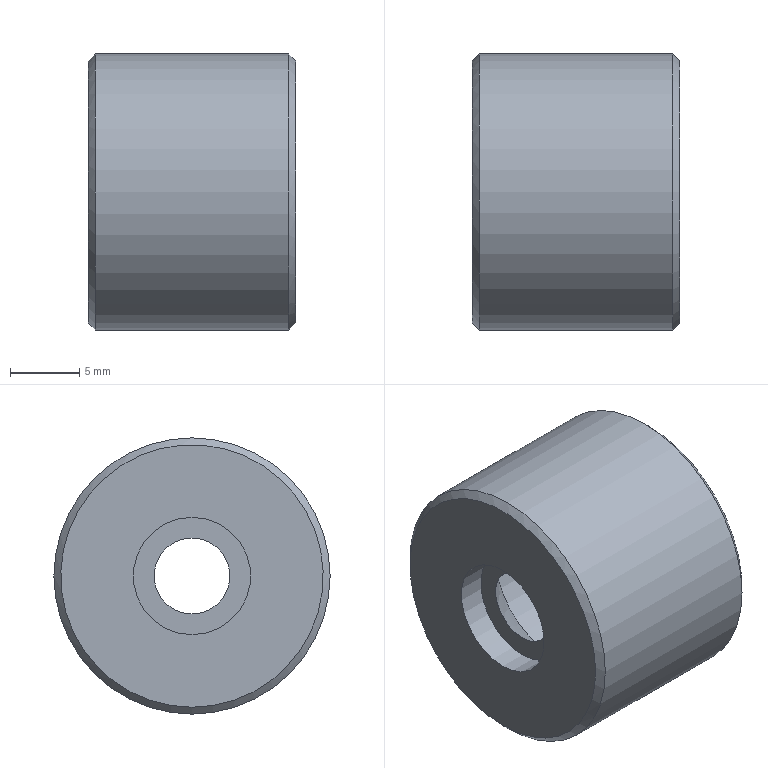Part | NX | features BREP 1 | 1 solid | 12 faces | box 15 x 20 x 20 mm | volume 3272 mm3 | cylinder 4 | plane 4 | cone 4 | commonest cylinder face diameters 5.5 x1 8.5 x1 12 x1 20 x1
STEP:
#1=CARTESIAN_POINT('',(2.015,0.,-2.75));
#2=VERTEX_POINT('',#1);
#3=CARTESIAN_POINT('',(2.015,0.,0.));
#4=DIRECTION('',(1.,0.,0.));
#5=DIRECTION('',(0.,0.,-1.));
#6=AXIS2_PLACEMENT_3D('',#3,#4,#5);
#7=CIRCLE('',#6,2.75);
#8=EDGE_CURVE('',#2,#2,#7,.T.);
#9=ORIENTED_EDGE('',*,*,#8,.T.);
#10=EDGE_LOOP('',(#9));
#11=FACE_BOUND('',#10,.T.);
#12=CARTESIAN_POINT('',(2.,0.,2.75));
#13=VERTEX_POINT('',#12);
#14=CARTESIAN_POINT('',(2.,0.,0.));
#15=DIRECTION('',(1.,0.,0.));
#16=DIRECTION('',(0.,0.,1.));
#17=AXIS2_PLACEMENT_3D('',#14,#15,#16);
#18=CIRCLE('',#17,2.75);
#19=EDGE_CURVE('',#13,#13,#18,.T.);
#20=ORIENTED_EDGE('',*,*,#19,.F.);
#21=EDGE_LOOP('',(#20));
#22=FACE_BOUND('',#21,.T.);
#23=CARTESIAN_POINT('',(5.,0.,0.));
#24=DIRECTION('',(1.,0.,0.));
#25=DIRECTION('',(0.,0.,1.));
#26=AXIS2_PLACEMENT_3D('',#23,#24,#25);
#27=CYLINDRICAL_SURFACE('',#26,2.75);
#28=ADVANCED_FACE('',(#11,#22),#27,.F.);
#29=CARTESIAN_POINT('',(0.,0.,4.25));
#30=VERTEX_POINT('',#29);
#31=CARTESIAN_POINT('',(0.,0.,0.));
#32=DIRECTION('',(-1.,0.,0.));
#33=DIRECTION('',(0.,0.,1.));
#34=AXIS2_PLACEMENT_3D('',#31,#32,#33);
#35=CIRCLE('',#34,4.25);
#36=EDGE_CURVE('',#30,#30,#35,.T.);
#37=ORIENTED_EDGE('',*,*,#36,.F.);
#38=EDGE_LOOP('',(#37));
#39=FACE_BOUND('',#38,.T.);
#40=CARTESIAN_POINT('',(0.,0.,-9.5));
#41=VERTEX_POINT('',#40);
#42=CARTESIAN_POINT('',(0.,0.,0.));
#43=DIRECTION('',(-1.,0.,0.));
#44=DIRECTION('',(0.,0.,-1.));
#45=AXIS2_PLACEMENT_3D('',#42,#43,#44);
#46=CIRCLE('',#45,9.5);
#47=EDGE_CURVE('',#41,#41,#46,.T.);
#48=ORIENTED_EDGE('',*,*,#47,.T.);
#49=EDGE_LOOP('',(#48));
#50=FACE_BOUND('',#49,.T.);
#51=CARTESIAN_POINT('',(0.,10.,0.));
#52=DIRECTION('',(1.,0.,0.));
#53=DIRECTION('',(0.,0.,1.));
#54=AXIS2_PLACEMENT_3D('',#51,#52,#53);
#55=PLANE('',#54);
#56=ADVANCED_FACE('',(#39,#50),#55,.F.);
#57=CARTESIAN_POINT('',(5.,0.,-5.735));
#58=VERTEX_POINT('',#57);
#59=CARTESIAN_POINT('',(5.,0.,0.));
#60=DIRECTION('',(1.,0.,0.));
#61=DIRECTION('',(0.,0.,-1.));
#62=AXIS2_PLACEMENT_3D('',#59,#60,#61);
#63=CIRCLE('',#62,5.735);
#64=EDGE_CURVE('',#58,#58,#63,.T.);
#65=ORIENTED_EDGE('',*,*,#64,.F.);
#66=EDGE_LOOP('',(#65));
#67=FACE_BOUND('',#66,.T.);
#68=CARTESIAN_POINT('',(5.,0.,6.));
#69=VERTEX_POINT('',#68);
#70=CARTESIAN_POINT('',(5.,0.,0.));
#71=DIRECTION('',(-1.,0.,0.));
#72=DIRECTION('',(0.,0.,1.));
#73=AXIS2_PLACEMENT_3D('',#70,#71,#72);
#74=CIRCLE('',#73,6.);
#75=EDGE_CURVE('',#69,#69,#74,.T.);
#76=ORIENTED_EDGE('',*,*,#75,.F.);
#77=EDGE_LOOP('',(#76));
#78=FACE_BOUND('',#77,.T.);
#79=CARTESIAN_POINT('',(5.,0.,0.));
#80=DIRECTION('',(-1.,0.,0.));
#81=DIRECTION('',(0.,0.,-1.));
#82=AXIS2_PLACEMENT_3D('',#79,#80,#81);
#83=PLANE('',#82);
#84=ADVANCED_FACE('',(#67,#78),#83,.F.);
#85=CARTESIAN_POINT('',(14.5,0.,6.));
#86=VERTEX_POINT('',#85);
#87=CARTESIAN_POINT('',(14.5,0.,0.));
#88=DIRECTION('',(1.,0.,0.));
#89=DIRECTION('',(0.,0.,1.));
#90=AXIS2_PLACEMENT_3D('',#87,#88,#89);
#91=CIRCLE('',#90,6.);
#92=EDGE_CURVE('',#86,#86,#91,.T.);
#93=ORIENTED_EDGE('',*,*,#92,.T.);
#94=EDGE_LOOP('',(#93));
#95=FACE_BOUND('',#94,.T.);
#96=ORIENTED_EDGE('',*,*,#75,.T.);
#97=EDGE_LOOP('',(#96));
#98=FACE_BOUND('',#97,.T.);
#99=CARTESIAN_POINT('',(0.,0.,0.));
#100=DIRECTION('',(-1.,0.,0.));
#101=DIRECTION('',(0.,0.,-1.));
#102=AXIS2_PLACEMENT_3D('',#99,#100,#101);
#103=CYLINDRICAL_SURFACE('',#102,6.);
#104=ADVANCED_FACE('',(#95,#98),#103,.F.);
#105=CARTESIAN_POINT('',(15.,0.,6.5));
#106=VERTEX_POINT('',#105);
#107=CARTESIAN_POINT('',(15.,0.,0.));
#108=DIRECTION('',(-1.,0.,0.));
#109=DIRECTION('',(0.,0.,1.));
#110=AXIS2_PLACEMENT_3D('',#107,#108,#109);
#111=CIRCLE('',#110,6.5);
#112=EDGE_CURVE('',#106,#106,#111,.T.);
#113=ORIENTED_EDGE('',*,*,#112,.T.);
#114=EDGE_LOOP('',(#113));
#115=FACE_BOUND('',#114,.T.);
#116=CARTESIAN_POINT('',(15.,0.,9.5));
#117=VERTEX_POINT('',#116);
#118=CARTESIAN_POINT('',(15.,0.,0.));
#119=DIRECTION('',(1.,0.,0.));
#120=DIRECTION('',(0.,0.,1.));
#121=AXIS2_PLACEMENT_3D('',#118,#119,#120);
#122=CIRCLE('',#121,9.5);
#123=EDGE_CURVE('',#117,#117,#122,.T.);
#124=ORIENTED_EDGE('',*,*,#123,.T.);
#125=EDGE_LOOP('',(#124));
#126=FACE_BOUND('',#125,.T.);
#127=CARTESIAN_POINT('',(15.,6.,0.));
#128=DIRECTION('',(-1.,0.,0.));
#129=DIRECTION('',(0.,0.,-1.));
#130=AXIS2_PLACEMENT_3D('',#127,#128,#129);
#131=PLANE('',#130);
#132=ADVANCED_FACE('',(#115,#126),#131,.F.);
#133=CARTESIAN_POINT('',(14.5,0.,10.));
#134=VERTEX_POINT('',#133);
#135=CARTESIAN_POINT('',(14.5,0.,0.));
#136=DIRECTION('',(-1.,0.,0.));
#137=DIRECTION('',(0.,0.,1.));
#138=AXIS2_PLACEMENT_3D('',#135,#136,#137);
#139=CIRCLE('',#138,10.);
#140=EDGE_CURVE('',#134,#134,#139,.T.);
#141=ORIENTED_EDGE('',*,*,#140,.T.);
#142=EDGE_LOOP('',(#141));
#143=FACE_BOUND('',#142,.T.);
#144=CARTESIAN_POINT('',(0.5,0.,-10.));
#145=VERTEX_POINT('',#144);
#146=CARTESIAN_POINT('',(0.5,0.,0.));
#147=DIRECTION('',(1.,0.,0.));
#148=DIRECTION('',(0.,0.,-1.));
#149=AXIS2_PLACEMENT_3D('',#146,#147,#148);
#150=CIRCLE('',#149,10.);
#151=EDGE_CURVE('',#145,#145,#150,.T.);
#152=ORIENTED_EDGE('',*,*,#151,.T.);
#153=EDGE_LOOP('',(#152));
#154=FACE_BOUND('',#153,.T.);
#155=CARTESIAN_POINT('',(0.,0.,0.));
#156=DIRECTION('',(-1.,0.,0.));
#157=DIRECTION('',(0.,0.,-1.));
#158=AXIS2_PLACEMENT_3D('',#155,#156,#157);
#159=CYLINDRICAL_SURFACE('',#158,10.);
#160=ADVANCED_FACE('',(#143,#154),#159,.T.);
#161=ORIENTED_EDGE('',*,*,#92,.F.);
#162=EDGE_LOOP('',(#161));
#163=FACE_BOUND('',#162,.T.);
#164=ORIENTED_EDGE('',*,*,#112,.F.);
#165=EDGE_LOOP('',(#164));
#166=FACE_BOUND('',#165,.T.);
#167=CARTESIAN_POINT('',(15.,0.,0.));
#168=DIRECTION('',(1.,0.,0.));
#169=DIRECTION('',(0.,0.,1.));
#170=AXIS2_PLACEMENT_3D('',#167,#168,#169);
#171=CONICAL_SURFACE('',#170,6.5,0.7854);
#172=ADVANCED_FACE('',(#163,#166),#171,.F.);
#173=ORIENTED_EDGE('',*,*,#123,.F.);
#174=EDGE_LOOP('',(#173));
#175=FACE_BOUND('',#174,.T.);
#176=ORIENTED_EDGE('',*,*,#140,.F.);
#177=EDGE_LOOP('',(#176));
#178=FACE_BOUND('',#177,.T.);
#179=CARTESIAN_POINT('',(14.5,0.,0.));
#180=DIRECTION('',(-1.,0.,0.));
#181=DIRECTION('',(0.,0.,-1.));
#182=AXIS2_PLACEMENT_3D('',#179,#180,#181);
#183=CONICAL_SURFACE('',#182,10.,0.7854);
#184=ADVANCED_FACE('',(#175,#178),#183,.T.);
#185=ORIENTED_EDGE('',*,*,#151,.F.);
#186=EDGE_LOOP('',(#185));
#187=FACE_BOUND('',#186,.T.);
#188=ORIENTED_EDGE('',*,*,#47,.F.);
#189=EDGE_LOOP('',(#188));
#190=FACE_BOUND('',#189,.T.);
#191=CARTESIAN_POINT('',(0.,0.,0.));
#192=DIRECTION('',(1.,0.,0.));
#193=DIRECTION('',(0.,0.,1.));
#194=AXIS2_PLACEMENT_3D('',#191,#192,#193);
#195=CONICAL_SURFACE('',#194,9.5,0.7854);
#196=ADVANCED_FACE('',(#187,#190),#195,.T.);
#197=ORIENTED_EDGE('',*,*,#8,.F.);
#198=EDGE_LOOP('',(#197));
#199=FACE_BOUND('',#198,.T.);
#200=ORIENTED_EDGE('',*,*,#64,.T.);
#201=EDGE_LOOP('',(#200));
#202=FACE_BOUND('',#201,.T.);
#203=CARTESIAN_POINT('',(5.,0.,0.));
#204=DIRECTION('',(1.,0.,0.));
#205=DIRECTION('',(0.,0.,1.));
#206=AXIS2_PLACEMENT_3D('',#203,#204,#205);
#207=CONICAL_SURFACE('',#206,5.735,0.7854);
#208=ADVANCED_FACE('',(#199,#202),#207,.F.);
#209=CARTESIAN_POINT('',(2.,0.,4.25));
#210=VERTEX_POINT('',#209);
#211=CARTESIAN_POINT('',(2.,0.,0.));
#212=DIRECTION('',(-1.,0.,0.));
#213=DIRECTION('',(0.,0.,1.));
#214=AXIS2_PLACEMENT_3D('',#211,#212,#213);
#215=CIRCLE('',#214,4.25);
#216=EDGE_CURVE('',#210,#210,#215,.T.);
#217=ORIENTED_EDGE('',*,*,#216,.T.);
#218=EDGE_LOOP('',(#217));
#219=FACE_BOUND('',#218,.T.);
#220=ORIENTED_EDGE('',*,*,#19,.T.);
#221=EDGE_LOOP('',(#220));
#222=FACE_BOUND('',#221,.T.);
#223=CARTESIAN_POINT('',(2.,0.,0.));
#224=DIRECTION('',(-1.,0.,0.));
#225=DIRECTION('',(0.,0.,-1.));
#226=AXIS2_PLACEMENT_3D('',#223,#224,#225);
#227=PLANE('',#226);
#228=ADVANCED_FACE('',(#219,#222),#227,.T.);
#229=ORIENTED_EDGE('',*,*,#216,.F.);
#230=EDGE_LOOP('',(#229));
#231=FACE_BOUND('',#230,.T.);
#232=ORIENTED_EDGE('',*,*,#36,.T.);
#233=EDGE_LOOP('',(#232));
#234=FACE_BOUND('',#233,.T.);
#235=CARTESIAN_POINT('',(2.,0.,0.));
#236=DIRECTION('',(-1.,0.,0.));
#237=DIRECTION('',(0.,0.,-1.));
#238=AXIS2_PLACEMENT_3D('',#235,#236,#237);
#239=CYLINDRICAL_SURFACE('',#238,4.25);
#240=ADVANCED_FACE('',(#231,#234),#239,.F.);
#241=CLOSED_SHELL('',(#28,#56,#84,#104,#132,#160,#172,#184,#196,#208,#228,#240));
#242=MANIFOLD_SOLID_BREP('',#241);
#243=(LENGTH_UNIT()NAMED_UNIT(*)SI_UNIT(.MILLI.,.METRE.));
#244=UNCERTAINTY_MEASURE_WITH_UNIT(LENGTH_MEASURE(0.00001),#243,'','');
#245=(NAMED_UNIT(*)PLANE_ANGLE_UNIT()SI_UNIT($,.RADIAN.));
#246=(NAMED_UNIT(*)SI_UNIT($,.STERADIAN.)SOLID_ANGLE_UNIT());
#247=(GEOMETRIC_REPRESENTATION_CONTEXT(3)GLOBAL_UNCERTAINTY_ASSIGNED_CONTEXT((#244))GLOBAL_UNIT_ASSIGNED_CONTEXT((#243,#245,#246))REPRESENTATION_CONTEXT('',''));
#248=ADVANCED_BREP_SHAPE_REPRESENTATION('',(#242),#247);